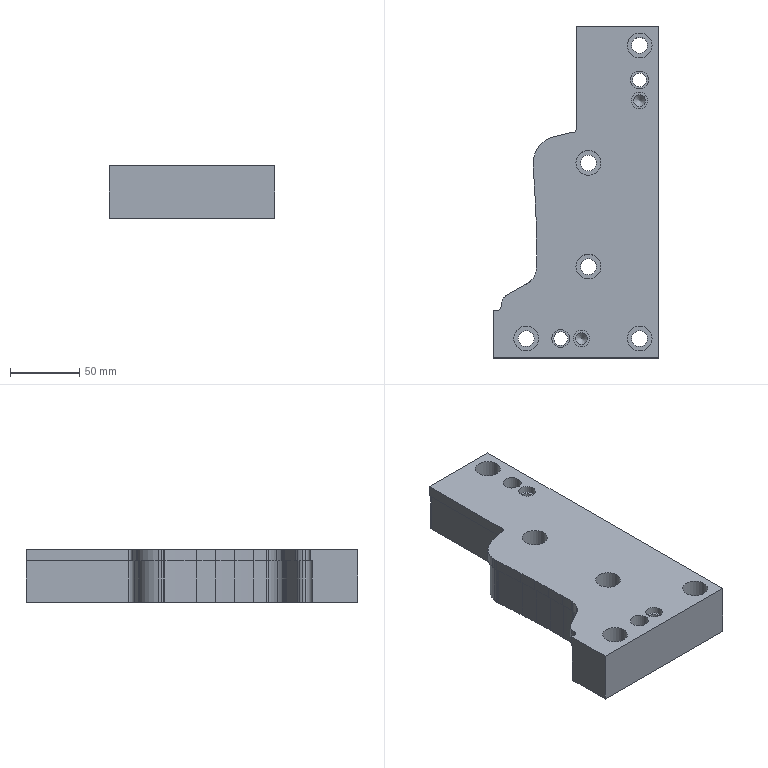Part | STEP file | lll_id4682_x_t | 1 solid | 93 faces | box 120 x 240 x 38 mm | volume 721958 mm3 | cylinder 69 | plane 22 | cone 2 | commonest cylinder face diameters 11.509 x5 18.008 x5 6 x3 13 x3 8.506 x2 9 x2